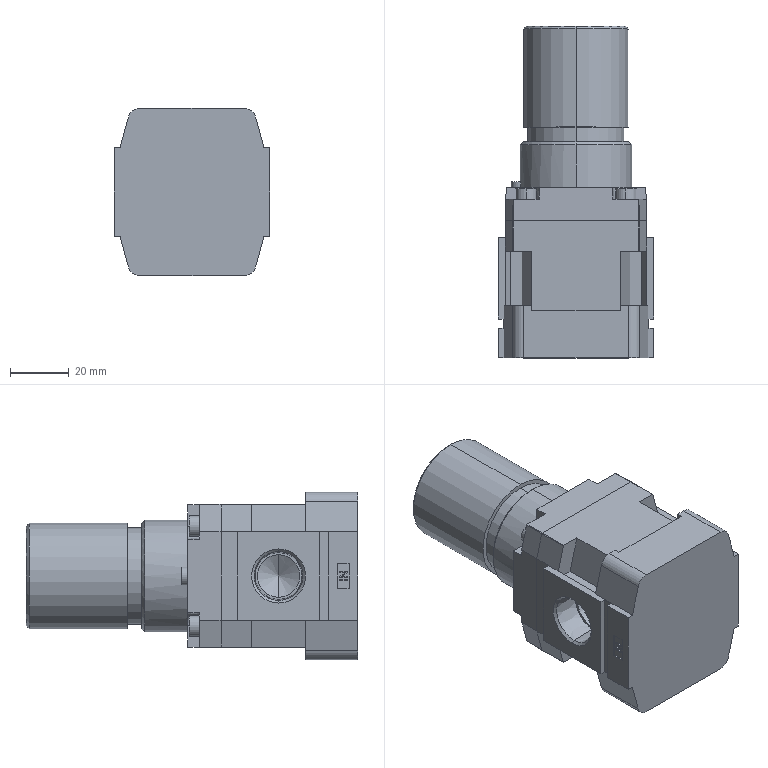Part | STEP file | AW30-03E_AW3020A Body_30 | 1 solid | 197 faces | box 53 x 113 x 57 mm | volume 188440 mm3 | plane 134 | cylinder 27 | cone 24 | spline 12 | commonest cylinder face diameters 7 x8 0.5 x4 8 x4 14.5 x4 33 x2 36 x2